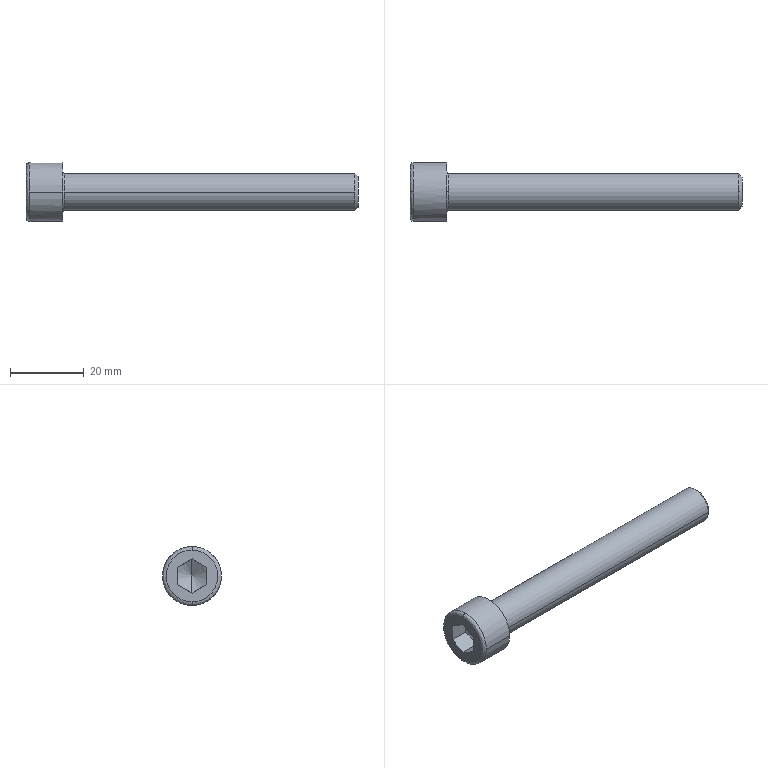Part | STEP file | Broached Socket Head Cap Screw - Metric M10x1.5 x 80 | 1 solid | 21 faces | box 90 x 16 x 16 mm | volume 7937 mm3 | plane 9 | spline 4 | cylinder 4 | cone 4 | commonest cylinder face diameters 10 x2 16 x2